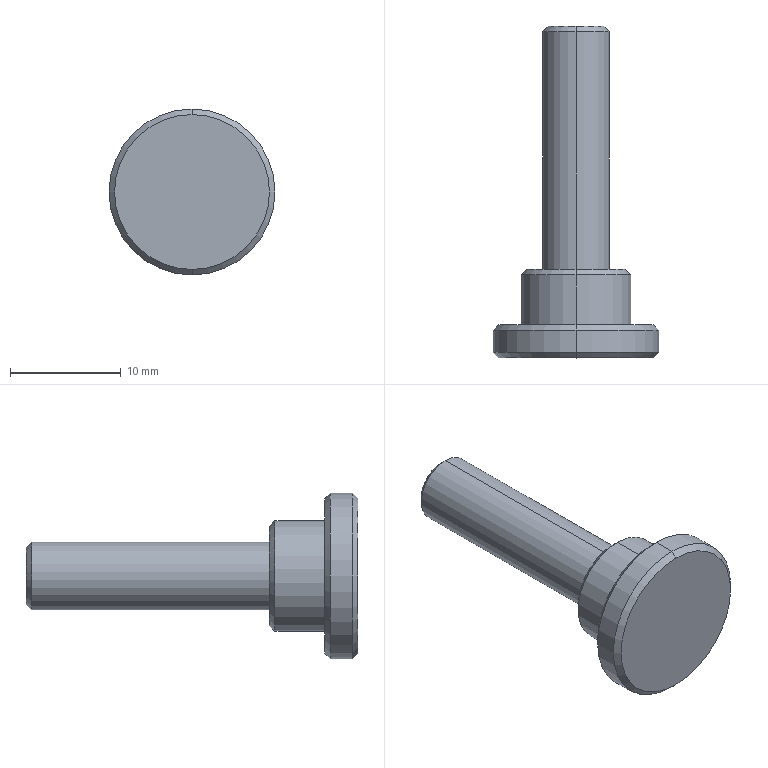Part | SolidWorks | features Chamfer 1, Revolution 1 | 1 solid | 18 faces | box 15 x 30 x 15 mm | volume 1548 mm3 | cone 8 | cylinder 6 | plane 4 | commonest cylinder face diameters 6.1 x2 10 x2 15 x2
STEP:
#1=CARTESIAN_POINT('',(0.,30.,2.55));
#2=VERTEX_POINT('',#1);
#3=CARTESIAN_POINT('',(0.,30.,-2.55));
#4=VERTEX_POINT('',#3);
#5=CARTESIAN_POINT('',(0.,30.,0.));
#6=DIRECTION('',(0.,1.,0.));
#7=DIRECTION('',(0.,0.,1.));
#8=AXIS2_PLACEMENT_3D('',#5,#6,#7);
#9=CIRCLE('',#8,2.55);
#10=EDGE_CURVE('',#2,#4,#9,.T.);
#11=ORIENTED_EDGE('',*,*,#10,.F.);
#12=CARTESIAN_POINT('',(0.,29.5,3.05));
#13=VERTEX_POINT('',#12);
#14=CARTESIAN_POINT('',(0.,29.5,3.05));
#15=DIRECTION('',(0.,-0.7071,0.7071));
#16=VECTOR('',#15,1000.);
#17=LINE('',#14,#16);
#18=EDGE_CURVE('',#2,#13,#17,.T.);
#19=ORIENTED_EDGE('',*,*,#18,.T.);
#20=CARTESIAN_POINT('',(0.,29.5,-3.05));
#21=VERTEX_POINT('',#20);
#22=CARTESIAN_POINT('',(0.,29.5,0.));
#23=DIRECTION('',(0.,-1.,0.));
#24=DIRECTION('',(0.,0.,1.));
#25=AXIS2_PLACEMENT_3D('',#22,#23,#24);
#26=CIRCLE('',#25,3.05);
#27=EDGE_CURVE('',#21,#13,#26,.T.);
#28=ORIENTED_EDGE('',*,*,#27,.F.);
#29=CARTESIAN_POINT('',(0.,29.5,-3.05));
#30=DIRECTION('',(0.,-0.7071,-0.7071));
#31=VECTOR('',#30,1000.);
#32=LINE('',#29,#31);
#33=EDGE_CURVE('',#4,#21,#32,.T.);
#34=ORIENTED_EDGE('',*,*,#33,.F.);
#35=EDGE_LOOP('',(#11,#19,#28,#34));
#36=FACE_OUTER_BOUND('',#35,.T.);
#37=CARTESIAN_POINT('',(0.,29.5,0.));
#38=DIRECTION('',(0.,-1.,0.));
#39=DIRECTION('',(0.,0.,-1.));
#40=AXIS2_PLACEMENT_3D('',#37,#38,#39);
#41=CONICAL_SURFACE('',#40,3.05,0.7854);
#42=ADVANCED_FACE('',(#36),#41,.T.);
#43=CARTESIAN_POINT('',(0.,8.,4.5));
#44=VERTEX_POINT('',#43);
#45=CARTESIAN_POINT('',(0.,8.,-4.5));
#46=VERTEX_POINT('',#45);
#47=CARTESIAN_POINT('',(0.,8.,0.));
#48=DIRECTION('',(0.,1.,0.));
#49=DIRECTION('',(0.,0.,1.));
#50=AXIS2_PLACEMENT_3D('',#47,#48,#49);
#51=CIRCLE('',#50,4.5);
#52=EDGE_CURVE('',#44,#46,#51,.T.);
#53=ORIENTED_EDGE('',*,*,#52,.F.);
#54=CARTESIAN_POINT('',(0.,7.5,5.));
#55=VERTEX_POINT('',#54);
#56=CARTESIAN_POINT('',(0.,7.5,5.));
#57=DIRECTION('',(0.,-0.7071,0.7071));
#58=VECTOR('',#57,1000.);
#59=LINE('',#56,#58);
#60=EDGE_CURVE('',#44,#55,#59,.T.);
#61=ORIENTED_EDGE('',*,*,#60,.T.);
#62=CARTESIAN_POINT('',(0.,7.5,-5.));
#63=VERTEX_POINT('',#62);
#64=CARTESIAN_POINT('',(0.,7.5,0.));
#65=DIRECTION('',(0.,-1.,0.));
#66=DIRECTION('',(0.,0.,1.));
#67=AXIS2_PLACEMENT_3D('',#64,#65,#66);
#68=CIRCLE('',#67,5.);
#69=EDGE_CURVE('',#63,#55,#68,.T.);
#70=ORIENTED_EDGE('',*,*,#69,.F.);
#71=CARTESIAN_POINT('',(0.,7.5,-5.));
#72=DIRECTION('',(0.,-0.7071,-0.7071));
#73=VECTOR('',#72,1000.);
#74=LINE('',#71,#73);
#75=EDGE_CURVE('',#46,#63,#74,.T.);
#76=ORIENTED_EDGE('',*,*,#75,.F.);
#77=EDGE_LOOP('',(#53,#61,#70,#76));
#78=FACE_OUTER_BOUND('',#77,.T.);
#79=CARTESIAN_POINT('',(0.,7.5,0.));
#80=DIRECTION('',(0.,-1.,0.));
#81=DIRECTION('',(0.,0.,-1.));
#82=AXIS2_PLACEMENT_3D('',#79,#80,#81);
#83=CONICAL_SURFACE('',#82,5.,0.7854);
#84=ADVANCED_FACE('',(#78),#83,.T.);
#85=CARTESIAN_POINT('',(0.,3.,7.));
#86=VERTEX_POINT('',#85);
#87=CARTESIAN_POINT('',(0.,3.,-7.));
#88=VERTEX_POINT('',#87);
#89=CARTESIAN_POINT('',(0.,3.,0.));
#90=DIRECTION('',(0.,1.,0.));
#91=DIRECTION('',(0.,0.,1.));
#92=AXIS2_PLACEMENT_3D('',#89,#90,#91);
#93=CIRCLE('',#92,7.);
#94=EDGE_CURVE('',#86,#88,#93,.T.);
#95=ORIENTED_EDGE('',*,*,#94,.F.);
#96=CARTESIAN_POINT('',(0.,2.5,7.5));
#97=VERTEX_POINT('',#96);
#98=CARTESIAN_POINT('',(0.,2.5,7.5));
#99=DIRECTION('',(0.,-0.7071,0.7071));
#100=VECTOR('',#99,1000.);
#101=LINE('',#98,#100);
#102=EDGE_CURVE('',#86,#97,#101,.T.);
#103=ORIENTED_EDGE('',*,*,#102,.T.);
#104=CARTESIAN_POINT('',(0.,2.5,-7.5));
#105=VERTEX_POINT('',#104);
#106=CARTESIAN_POINT('',(0.,2.5,0.));
#107=DIRECTION('',(0.,-1.,0.));
#108=DIRECTION('',(0.,0.,1.));
#109=AXIS2_PLACEMENT_3D('',#106,#107,#108);
#110=CIRCLE('',#109,7.5);
#111=EDGE_CURVE('',#105,#97,#110,.T.);
#112=ORIENTED_EDGE('',*,*,#111,.F.);
#113=CARTESIAN_POINT('',(0.,2.5,-7.5));
#114=DIRECTION('',(0.,-0.7071,-0.7071));
#115=VECTOR('',#114,1000.);
#116=LINE('',#113,#115);
#117=EDGE_CURVE('',#88,#105,#116,.T.);
#118=ORIENTED_EDGE('',*,*,#117,.F.);
#119=EDGE_LOOP('',(#95,#103,#112,#118));
#120=FACE_OUTER_BOUND('',#119,.T.);
#121=CARTESIAN_POINT('',(0.,2.5,0.));
#122=DIRECTION('',(0.,-1.,0.));
#123=DIRECTION('',(0.,0.,-1.));
#124=AXIS2_PLACEMENT_3D('',#121,#122,#123);
#125=CONICAL_SURFACE('',#124,7.5,0.7854);
#126=ADVANCED_FACE('',(#120),#125,.T.);
#127=CARTESIAN_POINT('',(0.,0.,-7.));
#128=VERTEX_POINT('',#127);
#129=CARTESIAN_POINT('',(0.,0.,7.));
#130=VERTEX_POINT('',#129);
#131=CARTESIAN_POINT('',(0.,0.,0.));
#132=DIRECTION('',(0.,-1.,0.));
#133=DIRECTION('',(0.,0.,-1.));
#134=AXIS2_PLACEMENT_3D('',#131,#132,#133);
#135=CIRCLE('',#134,7.);
#136=EDGE_CURVE('',#128,#130,#135,.T.);
#137=ORIENTED_EDGE('',*,*,#136,.F.);
#138=CARTESIAN_POINT('',(0.,0.5,-7.5));
#139=VERTEX_POINT('',#138);
#140=CARTESIAN_POINT('',(0.,0.,-7.));
#141=DIRECTION('',(0.,0.7071,-0.7071));
#142=VECTOR('',#141,1000.);
#143=LINE('',#140,#142);
#144=EDGE_CURVE('',#128,#139,#143,.T.);
#145=ORIENTED_EDGE('',*,*,#144,.T.);
#146=CARTESIAN_POINT('',(0.,0.5,7.5));
#147=VERTEX_POINT('',#146);
#148=CARTESIAN_POINT('',(0.,0.5,0.));
#149=DIRECTION('',(0.,1.,0.));
#150=DIRECTION('',(0.,0.,-1.));
#151=AXIS2_PLACEMENT_3D('',#148,#149,#150);
#152=CIRCLE('',#151,7.5);
#153=EDGE_CURVE('',#147,#139,#152,.T.);
#154=ORIENTED_EDGE('',*,*,#153,.F.);
#155=CARTESIAN_POINT('',(0.,0.,7.));
#156=DIRECTION('',(0.,0.7071,0.7071));
#157=VECTOR('',#156,1000.);
#158=LINE('',#155,#157);
#159=EDGE_CURVE('',#130,#147,#158,.T.);
#160=ORIENTED_EDGE('',*,*,#159,.F.);
#161=EDGE_LOOP('',(#137,#145,#154,#160));
#162=FACE_OUTER_BOUND('',#161,.T.);
#163=CARTESIAN_POINT('',(0.,0.,0.));
#164=DIRECTION('',(0.,1.,0.));
#165=DIRECTION('',(0.,0.,1.));
#166=AXIS2_PLACEMENT_3D('',#163,#164,#165);
#167=CONICAL_SURFACE('',#166,7.,0.7854);
#168=ADVANCED_FACE('',(#162),#167,.T.);
#169=ORIENTED_EDGE('',*,*,#111,.T.);
#170=CARTESIAN_POINT('',(0.,0.,7.5));
#171=DIRECTION('',(0.,-1.,0.));
#172=VECTOR('',#171,1000.);
#173=LINE('',#170,#172);
#174=EDGE_CURVE('',#97,#147,#173,.T.);
#175=ORIENTED_EDGE('',*,*,#174,.T.);
#176=ORIENTED_EDGE('',*,*,#153,.T.);
#177=CARTESIAN_POINT('',(0.,0.,-7.5));
#178=DIRECTION('',(0.,-1.,0.));
#179=VECTOR('',#178,1000.);
#180=LINE('',#177,#179);
#181=EDGE_CURVE('',#105,#139,#180,.T.);
#182=ORIENTED_EDGE('',*,*,#181,.F.);
#183=EDGE_LOOP('',(#169,#175,#176,#182));
#184=FACE_OUTER_BOUND('',#183,.T.);
#185=CARTESIAN_POINT('',(0.,0.,0.));
#186=DIRECTION('',(0.,-1.,0.));
#187=DIRECTION('',(0.,0.,-1.));
#188=AXIS2_PLACEMENT_3D('',#185,#186,#187);
#189=CYLINDRICAL_SURFACE('',#188,7.5);
#190=ADVANCED_FACE('',(#184),#189,.T.);
#191=ORIENTED_EDGE('',*,*,#69,.T.);
#192=CARTESIAN_POINT('',(0.,3.,5.));
#193=VERTEX_POINT('',#192);
#194=CARTESIAN_POINT('',(0.,0.,5.));
#195=DIRECTION('',(0.,-1.,0.));
#196=VECTOR('',#195,1000.);
#197=LINE('',#194,#196);
#198=EDGE_CURVE('',#55,#193,#197,.T.);
#199=ORIENTED_EDGE('',*,*,#198,.T.);
#200=CARTESIAN_POINT('',(0.,3.,-5.));
#201=VERTEX_POINT('',#200);
#202=CARTESIAN_POINT('',(0.,3.,0.));
#203=DIRECTION('',(0.,-1.,0.));
#204=DIRECTION('',(0.,0.,-1.));
#205=AXIS2_PLACEMENT_3D('',#202,#203,#204);
#206=CIRCLE('',#205,5.);
#207=EDGE_CURVE('',#201,#193,#206,.T.);
#208=ORIENTED_EDGE('',*,*,#207,.F.);
#209=CARTESIAN_POINT('',(0.,0.,-5.));
#210=DIRECTION('',(0.,-1.,0.));
#211=VECTOR('',#210,1000.);
#212=LINE('',#209,#211);
#213=EDGE_CURVE('',#63,#201,#212,.T.);
#214=ORIENTED_EDGE('',*,*,#213,.F.);
#215=EDGE_LOOP('',(#191,#199,#208,#214));
#216=FACE_OUTER_BOUND('',#215,.T.);
#217=CARTESIAN_POINT('',(0.,0.,0.));
#218=DIRECTION('',(0.,-1.,0.));
#219=DIRECTION('',(0.,0.,-1.));
#220=AXIS2_PLACEMENT_3D('',#217,#218,#219);
#221=CYLINDRICAL_SURFACE('',#220,5.);
#222=ADVANCED_FACE('',(#216),#221,.T.);
#223=ORIENTED_EDGE('',*,*,#27,.T.);
#224=CARTESIAN_POINT('',(0.,8.,3.05));
#225=VERTEX_POINT('',#224);
#226=CARTESIAN_POINT('',(0.,0.,3.05));
#227=DIRECTION('',(0.,-1.,0.));
#228=VECTOR('',#227,1000.);
#229=LINE('',#226,#228);
#230=EDGE_CURVE('',#13,#225,#229,.T.);
#231=ORIENTED_EDGE('',*,*,#230,.T.);
#232=CARTESIAN_POINT('',(0.,8.,-3.05));
#233=VERTEX_POINT('',#232);
#234=CARTESIAN_POINT('',(0.,8.,0.));
#235=DIRECTION('',(0.,-1.,0.));
#236=DIRECTION('',(0.,0.,-1.));
#237=AXIS2_PLACEMENT_3D('',#234,#235,#236);
#238=CIRCLE('',#237,3.05);
#239=EDGE_CURVE('',#233,#225,#238,.T.);
#240=ORIENTED_EDGE('',*,*,#239,.F.);
#241=CARTESIAN_POINT('',(0.,0.,-3.05));
#242=DIRECTION('',(0.,-1.,0.));
#243=VECTOR('',#242,1000.);
#244=LINE('',#241,#243);
#245=EDGE_CURVE('',#21,#233,#244,.T.);
#246=ORIENTED_EDGE('',*,*,#245,.F.);
#247=EDGE_LOOP('',(#223,#231,#240,#246));
#248=FACE_OUTER_BOUND('',#247,.T.);
#249=CARTESIAN_POINT('',(0.,0.,0.));
#250=DIRECTION('',(0.,-1.,0.));
#251=DIRECTION('',(0.,0.,-1.));
#252=AXIS2_PLACEMENT_3D('',#249,#250,#251);
#253=CYLINDRICAL_SURFACE('',#252,3.05);
#254=ADVANCED_FACE('',(#248),#253,.T.);
#255=CARTESIAN_POINT('',(0.,30.,0.));
#256=DIRECTION('',(0.,1.,0.));
#257=DIRECTION('',(0.,0.,1.));
#258=AXIS2_PLACEMENT_3D('',#255,#256,#257);
#259=CIRCLE('',#258,2.55);
#260=EDGE_CURVE('',#4,#2,#259,.T.);
#261=ORIENTED_EDGE('',*,*,#260,.T.);
#262=ORIENTED_EDGE('',*,*,#10,.T.);
#263=EDGE_LOOP('',(#261,#262));
#264=FACE_OUTER_BOUND('',#263,.T.);
#265=CARTESIAN_POINT('',(0.,30.,0.));
#266=DIRECTION('',(0.,1.,0.));
#267=DIRECTION('',(0.,0.,1.));
#268=AXIS2_PLACEMENT_3D('',#265,#266,#267);
#269=PLANE('',#268);
#270=ADVANCED_FACE('',(#264),#269,.T.);
#271=ORIENTED_EDGE('',*,*,#230,.F.);
#272=CARTESIAN_POINT('',(0.,29.5,0.));
#273=DIRECTION('',(0.,-1.,0.));
#274=DIRECTION('',(0.,0.,1.));
#275=AXIS2_PLACEMENT_3D('',#272,#273,#274);
#276=CIRCLE('',#275,3.05);
#277=EDGE_CURVE('',#13,#21,#276,.T.);
#278=ORIENTED_EDGE('',*,*,#277,.T.);
#279=ORIENTED_EDGE('',*,*,#245,.T.);
#280=CARTESIAN_POINT('',(0.,8.,0.));
#281=DIRECTION('',(0.,-1.,0.));
#282=DIRECTION('',(0.,0.,-1.));
#283=AXIS2_PLACEMENT_3D('',#280,#281,#282);
#284=CIRCLE('',#283,3.05);
#285=EDGE_CURVE('',#225,#233,#284,.T.);
#286=ORIENTED_EDGE('',*,*,#285,.F.);
#287=EDGE_LOOP('',(#271,#278,#279,#286));
#288=FACE_OUTER_BOUND('',#287,.T.);
#289=CARTESIAN_POINT('',(0.,0.,0.));
#290=DIRECTION('',(0.,-1.,0.));
#291=DIRECTION('',(0.,0.,-1.));
#292=AXIS2_PLACEMENT_3D('',#289,#290,#291);
#293=CYLINDRICAL_SURFACE('',#292,3.05);
#294=ADVANCED_FACE('',(#288),#293,.T.);
#295=CARTESIAN_POINT('',(0.,8.,0.));
#296=DIRECTION('',(0.,1.,0.));
#297=DIRECTION('',(0.,0.,1.));
#298=AXIS2_PLACEMENT_3D('',#295,#296,#297);
#299=CIRCLE('',#298,4.5);
#300=EDGE_CURVE('',#46,#44,#299,.T.);
#301=ORIENTED_EDGE('',*,*,#300,.T.);
#302=ORIENTED_EDGE('',*,*,#52,.T.);
#303=EDGE_LOOP('',(#301,#302));
#304=FACE_OUTER_BOUND('',#303,.T.);
#305=ORIENTED_EDGE('',*,*,#239,.T.);
#306=ORIENTED_EDGE('',*,*,#285,.T.);
#307=EDGE_LOOP('',(#305,#306));
#308=FACE_BOUND('',#307,.T.);
#309=CARTESIAN_POINT('',(0.,8.,-3.05));
#310=DIRECTION('',(0.,1.,0.));
#311=DIRECTION('',(0.,0.,1.));
#312=AXIS2_PLACEMENT_3D('',#309,#310,#311);
#313=PLANE('',#312);
#314=ADVANCED_FACE('',(#304,#308),#313,.T.);
#315=ORIENTED_EDGE('',*,*,#198,.F.);
#316=CARTESIAN_POINT('',(0.,7.5,0.));
#317=DIRECTION('',(0.,-1.,0.));
#318=DIRECTION('',(0.,0.,1.));
#319=AXIS2_PLACEMENT_3D('',#316,#317,#318);
#320=CIRCLE('',#319,5.);
#321=EDGE_CURVE('',#55,#63,#320,.T.);
#322=ORIENTED_EDGE('',*,*,#321,.T.);
#323=ORIENTED_EDGE('',*,*,#213,.T.);
#324=CARTESIAN_POINT('',(0.,3.,0.));
#325=DIRECTION('',(0.,-1.,0.));
#326=DIRECTION('',(0.,0.,-1.));
#327=AXIS2_PLACEMENT_3D('',#324,#325,#326);
#328=CIRCLE('',#327,5.);
#329=EDGE_CURVE('',#193,#201,#328,.T.);
#330=ORIENTED_EDGE('',*,*,#329,.F.);
#331=EDGE_LOOP('',(#315,#322,#323,#330));
#332=FACE_OUTER_BOUND('',#331,.T.);
#333=CARTESIAN_POINT('',(0.,0.,0.));
#334=DIRECTION('',(0.,-1.,0.));
#335=DIRECTION('',(0.,0.,-1.));
#336=AXIS2_PLACEMENT_3D('',#333,#334,#335);
#337=CYLINDRICAL_SURFACE('',#336,5.);
#338=ADVANCED_FACE('',(#332),#337,.T.);
#339=CARTESIAN_POINT('',(0.,3.,0.));
#340=DIRECTION('',(0.,1.,0.));
#341=DIRECTION('',(0.,0.,1.));
#342=AXIS2_PLACEMENT_3D('',#339,#340,#341);
#343=CIRCLE('',#342,7.);
#344=EDGE_CURVE('',#88,#86,#343,.T.);
#345=ORIENTED_EDGE('',*,*,#344,.T.);
#346=ORIENTED_EDGE('',*,*,#94,.T.);
#347=EDGE_LOOP('',(#345,#346));
#348=FACE_OUTER_BOUND('',#347,.T.);
#349=ORIENTED_EDGE('',*,*,#207,.T.);
#350=ORIENTED_EDGE('',*,*,#329,.T.);
#351=EDGE_LOOP('',(#349,#350));
#352=FACE_BOUND('',#351,.T.);
#353=CARTESIAN_POINT('',(0.,3.,-5.));
#354=DIRECTION('',(0.,1.,0.));
#355=DIRECTION('',(0.,0.,1.));
#356=AXIS2_PLACEMENT_3D('',#353,#354,#355);
#357=PLANE('',#356);
#358=ADVANCED_FACE('',(#348,#352),#357,.T.);
#359=ORIENTED_EDGE('',*,*,#174,.F.);
#360=CARTESIAN_POINT('',(0.,2.5,0.));
#361=DIRECTION('',(0.,-1.,0.));
#362=DIRECTION('',(0.,0.,1.));
#363=AXIS2_PLACEMENT_3D('',#360,#361,#362);
#364=CIRCLE('',#363,7.5);
#365=EDGE_CURVE('',#97,#105,#364,.T.);
#366=ORIENTED_EDGE('',*,*,#365,.T.);
#367=ORIENTED_EDGE('',*,*,#181,.T.);
#368=CARTESIAN_POINT('',(0.,0.5,0.));
#369=DIRECTION('',(0.,1.,0.));
#370=DIRECTION('',(0.,0.,-1.));
#371=AXIS2_PLACEMENT_3D('',#368,#369,#370);
#372=CIRCLE('',#371,7.5);
#373=EDGE_CURVE('',#139,#147,#372,.T.);
#374=ORIENTED_EDGE('',*,*,#373,.T.);
#375=EDGE_LOOP('',(#359,#366,#367,#374));
#376=FACE_OUTER_BOUND('',#375,.T.);
#377=CARTESIAN_POINT('',(0.,0.,0.));
#378=DIRECTION('',(0.,-1.,0.));
#379=DIRECTION('',(0.,0.,-1.));
#380=AXIS2_PLACEMENT_3D('',#377,#378,#379);
#381=CYLINDRICAL_SURFACE('',#380,7.5);
#382=ADVANCED_FACE('',(#376),#381,.T.);
#383=CARTESIAN_POINT('',(0.,0.,0.));
#384=DIRECTION('',(0.,-1.,0.));
#385=DIRECTION('',(0.,0.,-1.));
#386=AXIS2_PLACEMENT_3D('',#383,#384,#385);
#387=CIRCLE('',#386,7.);
#388=EDGE_CURVE('',#130,#128,#387,.T.);
#389=ORIENTED_EDGE('',*,*,#388,.T.);
#390=ORIENTED_EDGE('',*,*,#136,.T.);
#391=EDGE_LOOP('',(#389,#390));
#392=FACE_OUTER_BOUND('',#391,.T.);
#393=CARTESIAN_POINT('',(0.,0.,-7.5));
#394=DIRECTION('',(0.,-1.,0.));
#395=DIRECTION('',(0.,0.,-1.));
#396=AXIS2_PLACEMENT_3D('',#393,#394,#395);
#397=PLANE('',#396);
#398=ADVANCED_FACE('',(#392),#397,.T.);
#399=ORIENTED_EDGE('',*,*,#144,.F.);
#400=ORIENTED_EDGE('',*,*,#388,.F.);
#401=ORIENTED_EDGE('',*,*,#159,.T.);
#402=ORIENTED_EDGE('',*,*,#373,.F.);
#403=EDGE_LOOP('',(#399,#400,#401,#402));
#404=FACE_OUTER_BOUND('',#403,.T.);
#405=CARTESIAN_POINT('',(0.,0.,0.));
#406=DIRECTION('',(0.,1.,0.));
#407=DIRECTION('',(0.,0.,1.));
#408=AXIS2_PLACEMENT_3D('',#405,#406,#407);
#409=CONICAL_SURFACE('',#408,7.,0.7854);
#410=ADVANCED_FACE('',(#404),#409,.T.);
#411=ORIENTED_EDGE('',*,*,#102,.F.);
#412=ORIENTED_EDGE('',*,*,#344,.F.);
#413=ORIENTED_EDGE('',*,*,#117,.T.);
#414=ORIENTED_EDGE('',*,*,#365,.F.);
#415=EDGE_LOOP('',(#411,#412,#413,#414));
#416=FACE_OUTER_BOUND('',#415,.T.);
#417=CARTESIAN_POINT('',(0.,2.5,0.));
#418=DIRECTION('',(0.,-1.,0.));
#419=DIRECTION('',(0.,0.,-1.));
#420=AXIS2_PLACEMENT_3D('',#417,#418,#419);
#421=CONICAL_SURFACE('',#420,7.5,0.7854);
#422=ADVANCED_FACE('',(#416),#421,.T.);
#423=ORIENTED_EDGE('',*,*,#60,.F.);
#424=ORIENTED_EDGE('',*,*,#300,.F.);
#425=ORIENTED_EDGE('',*,*,#75,.T.);
#426=ORIENTED_EDGE('',*,*,#321,.F.);
#427=EDGE_LOOP('',(#423,#424,#425,#426));
#428=FACE_OUTER_BOUND('',#427,.T.);
#429=CARTESIAN_POINT('',(0.,7.5,0.));
#430=DIRECTION('',(0.,-1.,0.));
#431=DIRECTION('',(0.,0.,-1.));
#432=AXIS2_PLACEMENT_3D('',#429,#430,#431);
#433=CONICAL_SURFACE('',#432,5.,0.7854);
#434=ADVANCED_FACE('',(#428),#433,.T.);
#435=ORIENTED_EDGE('',*,*,#18,.F.);
#436=ORIENTED_EDGE('',*,*,#260,.F.);
#437=ORIENTED_EDGE('',*,*,#33,.T.);
#438=ORIENTED_EDGE('',*,*,#277,.F.);
#439=EDGE_LOOP('',(#435,#436,#437,#438));
#440=FACE_OUTER_BOUND('',#439,.T.);
#441=CARTESIAN_POINT('',(0.,29.5,0.));
#442=DIRECTION('',(0.,-1.,0.));
#443=DIRECTION('',(0.,0.,-1.));
#444=AXIS2_PLACEMENT_3D('',#441,#442,#443);
#445=CONICAL_SURFACE('',#444,3.05,0.7854);
#446=ADVANCED_FACE('',(#440),#445,.T.);
#447=CLOSED_SHELL('',(#42,#84,#126,#168,#190,#222,#254,#270,#294,#314,#338,#358,#382,#398,#410,#422,#434,#446));
#448=MANIFOLD_SOLID_BREP('',#447);
#449=CARTESIAN_POINT('',(0.,0.,0.));
#450=DIRECTION('',(0.,0.,1.));
#451=DIRECTION('',(1.,0.,0.));
#452=AXIS2_PLACEMENT_3D('',#449,#450,#451);
#453=(LENGTH_UNIT()NAMED_UNIT(*)SI_UNIT(.MILLI.,.METRE.));
#454=UNCERTAINTY_MEASURE_WITH_UNIT(LENGTH_MEASURE(0.00001),#453,'','');
#455=(NAMED_UNIT(*)PLANE_ANGLE_UNIT()SI_UNIT($,.RADIAN.));
#456=(NAMED_UNIT(*)SI_UNIT($,.STERADIAN.)SOLID_ANGLE_UNIT());
#457=(GEOMETRIC_REPRESENTATION_CONTEXT(3)GLOBAL_UNCERTAINTY_ASSIGNED_CONTEXT((#454))GLOBAL_UNIT_ASSIGNED_CONTEXT((#453,#455,#456))REPRESENTATION_CONTEXT('',''));
#458=ADVANCED_BREP_SHAPE_REPRESENTATION('',(#448,#452),#457);